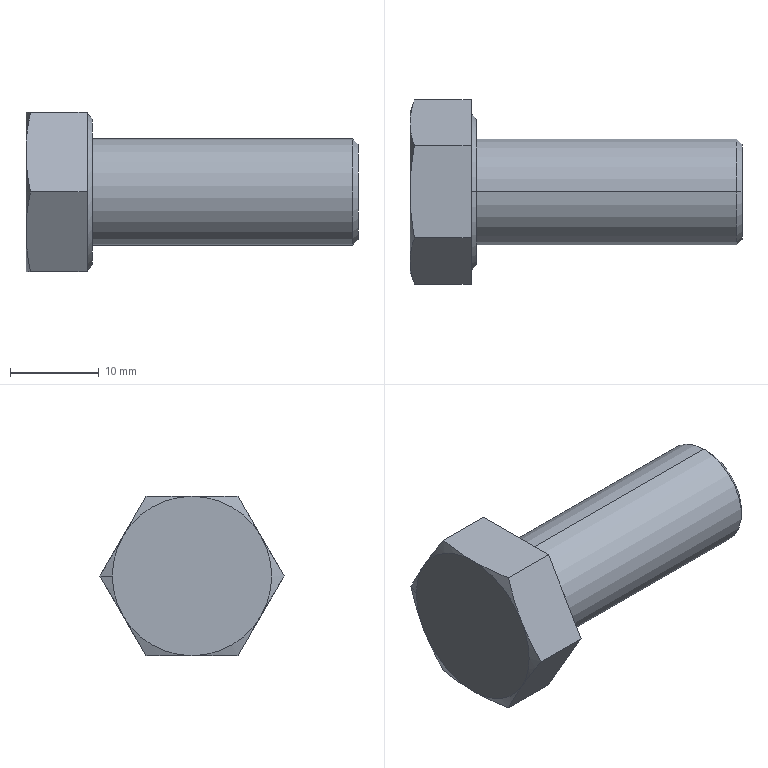Part | STEP file | hex head bolts-full thread grade c gb_GB_FASTENER_BOLT_HHBFTC M12X30-S | 1 solid | 23 faces | box 37.5 x 20.785 x 18 mm | volume 5456 mm3 | cone 11 | plane 10 | cylinder 2 | commonest cylinder face diameters 12 x2
STEP:
#1=CARTESIAN_POINT('',(36.9,0.,6.));
#2=VERTEX_POINT('',#1);
#3=CARTESIAN_POINT('',(36.9,0.,-6.));
#4=VERTEX_POINT('',#3);
#5=CARTESIAN_POINT('',(36.9,0.,0.));
#6=DIRECTION('',(-1.,0.,0.));
#7=DIRECTION('',(0.,0.,1.));
#8=AXIS2_PLACEMENT_3D('',#5,#6,#7);
#9=CIRCLE('',#8,6.);
#10=EDGE_CURVE('',#2,#4,#9,.T.);
#11=ORIENTED_EDGE('',*,*,#10,.T.);
#12=CARTESIAN_POINT('',(7.5,0.,-6.));
#13=VERTEX_POINT('',#12);
#14=CARTESIAN_POINT('',(37.5,0.,-6.));
#15=DIRECTION('',(-1.,0.,0.));
#16=VECTOR('',#15,1000.);
#17=LINE('',#14,#16);
#18=EDGE_CURVE('',#4,#13,#17,.T.);
#19=ORIENTED_EDGE('',*,*,#18,.T.);
#20=CARTESIAN_POINT('',(7.5,0.,6.));
#21=VERTEX_POINT('',#20);
#22=CARTESIAN_POINT('',(7.5,0.,0.));
#23=DIRECTION('',(1.,0.,0.));
#24=DIRECTION('',(0.,0.,1.));
#25=AXIS2_PLACEMENT_3D('',#22,#23,#24);
#26=CIRCLE('',#25,6.);
#27=EDGE_CURVE('',#13,#21,#26,.T.);
#28=ORIENTED_EDGE('',*,*,#27,.T.);
#29=CARTESIAN_POINT('',(37.5,0.,6.));
#30=DIRECTION('',(-1.,0.,0.));
#31=VECTOR('',#30,1000.);
#32=LINE('',#29,#31);
#33=EDGE_CURVE('',#2,#21,#32,.T.);
#34=ORIENTED_EDGE('',*,*,#33,.F.);
#35=EDGE_LOOP('',(#11,#19,#28,#34));
#36=FACE_OUTER_BOUND('',#35,.T.);
#37=CARTESIAN_POINT('',(37.5,0.,0.));
#38=DIRECTION('',(-1.,0.,0.));
#39=DIRECTION('',(0.,0.,1.));
#40=AXIS2_PLACEMENT_3D('',#37,#38,#39);
#41=CYLINDRICAL_SURFACE('',#40,6.);
#42=ADVANCED_FACE('',(#36),#41,.T.);
#43=CARTESIAN_POINT('',(37.5,0.,5.4));
#44=VERTEX_POINT('',#43);
#45=CARTESIAN_POINT('',(37.5,0.,-5.4));
#46=VERTEX_POINT('',#45);
#47=CARTESIAN_POINT('',(37.5,0.,0.));
#48=DIRECTION('',(-1.,0.,0.));
#49=DIRECTION('',(0.,0.,1.));
#50=AXIS2_PLACEMENT_3D('',#47,#48,#49);
#51=CIRCLE('',#50,5.4);
#52=EDGE_CURVE('',#44,#46,#51,.T.);
#53=ORIENTED_EDGE('',*,*,#52,.T.);
#54=CARTESIAN_POINT('',(36.9,0.,-6.));
#55=DIRECTION('',(-0.7071,0.,-0.7071));
#56=VECTOR('',#55,1000.);
#57=LINE('',#54,#56);
#58=EDGE_CURVE('',#46,#4,#57,.T.);
#59=ORIENTED_EDGE('',*,*,#58,.T.);
#60=ORIENTED_EDGE('',*,*,#10,.F.);
#61=CARTESIAN_POINT('',(36.9,0.,6.));
#62=DIRECTION('',(-0.7071,0.,0.7071));
#63=VECTOR('',#62,1000.);
#64=LINE('',#61,#63);
#65=EDGE_CURVE('',#44,#2,#64,.T.);
#66=ORIENTED_EDGE('',*,*,#65,.F.);
#67=EDGE_LOOP('',(#53,#59,#60,#66));
#68=FACE_OUTER_BOUND('',#67,.T.);
#69=CARTESIAN_POINT('',(36.9,0.,0.));
#70=DIRECTION('',(-1.,0.,0.));
#71=DIRECTION('',(0.,0.,1.));
#72=AXIS2_PLACEMENT_3D('',#69,#70,#71);
#73=CONICAL_SURFACE('',#72,6.,0.7854);
#74=ADVANCED_FACE('',(#68),#73,.T.);
#75=CARTESIAN_POINT('',(7.5,0.,8.235));
#76=VERTEX_POINT('',#75);
#77=CARTESIAN_POINT('',(7.5,0.,-8.235));
#78=VERTEX_POINT('',#77);
#79=CARTESIAN_POINT('',(7.5,0.,0.));
#80=DIRECTION('',(-1.,0.,0.));
#81=DIRECTION('',(0.,0.,1.));
#82=AXIS2_PLACEMENT_3D('',#79,#80,#81);
#83=CIRCLE('',#82,8.235);
#84=EDGE_CURVE('',#76,#78,#83,.T.);
#85=ORIENTED_EDGE('',*,*,#84,.T.);
#86=CARTESIAN_POINT('',(6.9,0.,-8.835));
#87=VERTEX_POINT('',#86);
#88=CARTESIAN_POINT('',(6.9,0.,-8.835));
#89=DIRECTION('',(-0.7071,0.,-0.7071));
#90=VECTOR('',#89,1000.);
#91=LINE('',#88,#90);
#92=EDGE_CURVE('',#78,#87,#91,.T.);
#93=ORIENTED_EDGE('',*,*,#92,.T.);
#94=CARTESIAN_POINT('',(6.9,0.,8.835));
#95=VERTEX_POINT('',#94);
#96=CARTESIAN_POINT('',(6.9,0.,0.));
#97=DIRECTION('',(1.,0.,0.));
#98=DIRECTION('',(0.,0.,1.));
#99=AXIS2_PLACEMENT_3D('',#96,#97,#98);
#100=CIRCLE('',#99,8.835);
#101=EDGE_CURVE('',#87,#95,#100,.T.);
#102=ORIENTED_EDGE('',*,*,#101,.T.);
#103=CARTESIAN_POINT('',(6.9,0.,8.835));
#104=DIRECTION('',(-0.7071,0.,0.7071));
#105=VECTOR('',#104,1000.);
#106=LINE('',#103,#105);
#107=EDGE_CURVE('',#76,#95,#106,.T.);
#108=ORIENTED_EDGE('',*,*,#107,.F.);
#109=EDGE_LOOP('',(#85,#93,#102,#108));
#110=FACE_OUTER_BOUND('',#109,.T.);
#111=CARTESIAN_POINT('',(6.9,0.,0.));
#112=DIRECTION('',(-1.,0.,0.));
#113=DIRECTION('',(0.,0.,1.));
#114=AXIS2_PLACEMENT_3D('',#111,#112,#113);
#115=CONICAL_SURFACE('',#114,8.835,0.7854);
#116=ADVANCED_FACE('',(#110),#115,.T.);
#117=CARTESIAN_POINT('',(0.,7.794,-4.5));
#118=VERTEX_POINT('',#117);
#119=CARTESIAN_POINT('',(0.,9.,0.));
#120=VERTEX_POINT('',#119);
#121=CARTESIAN_POINT('',(0.,0.,0.));
#122=DIRECTION('',(1.,0.,0.));
#123=DIRECTION('',(0.,1.,0.));
#124=AXIS2_PLACEMENT_3D('',#121,#122,#123);
#125=CIRCLE('',#124,9.);
#126=EDGE_CURVE('',#118,#120,#125,.T.);
#127=ORIENTED_EDGE('',*,*,#126,.T.);
#128=CARTESIAN_POINT('',(0.5068,10.392,0.));
#129=VERTEX_POINT('',#128);
#130=CARTESIAN_POINT('',(0.5098,10.401,0.));
#131=DIRECTION('',(0.342,0.9397,0.));
#132=VECTOR('',#131,1000.);
#133=LINE('',#130,#132);
#134=EDGE_CURVE('',#120,#129,#133,.T.);
#135=ORIENTED_EDGE('',*,*,#134,.T.);
#136=CARTESIAN_POINT('',(0.5068,10.392,0.));
#137=CARTESIAN_POINT('',(0.3504,9.963,-0.7439));
#138=CARTESIAN_POINT('',(0.2227,9.532,-1.49));
#139=CARTESIAN_POINT('',(0.04718,8.666,-2.99));
#140=CARTESIAN_POINT('',(0.,8.231,-3.743));
#141=CARTESIAN_POINT('',(0.,7.794,-4.5));
#142=B_SPLINE_CURVE_WITH_KNOTS('',3,(#136,#137,#138,#139,#140,#141),.UNSPECIFIED.,.F.,.F.,(4,2,4),(0.,0.00261,0.005221),.UNSPECIFIED.);
#143=EDGE_CURVE('',#129,#118,#142,.T.);
#144=ORIENTED_EDGE('',*,*,#143,.T.);
#145=EDGE_LOOP('',(#127,#135,#144));
#146=FACE_OUTER_BOUND('',#145,.T.);
#147=CARTESIAN_POINT('',(0.5098,0.,0.));
#148=DIRECTION('',(1.,0.,0.));
#149=DIRECTION('',(0.,1.,0.));
#150=AXIS2_PLACEMENT_3D('',#147,#148,#149);
#151=CONICAL_SURFACE('',#150,10.401,1.222);
#152=ADVANCED_FACE('',(#146),#151,.T.);
#153=ORIENTED_EDGE('',*,*,#18,.F.);
#154=CARTESIAN_POINT('',(36.9,0.,0.));
#155=DIRECTION('',(-1.,0.,0.));
#156=DIRECTION('',(0.,0.,1.));
#157=AXIS2_PLACEMENT_3D('',#154,#155,#156);
#158=CIRCLE('',#157,6.);
#159=EDGE_CURVE('',#4,#2,#158,.T.);
#160=ORIENTED_EDGE('',*,*,#159,.T.);
#161=ORIENTED_EDGE('',*,*,#33,.T.);
#162=CARTESIAN_POINT('',(7.5,0.,0.));
#163=DIRECTION('',(1.,0.,0.));
#164=DIRECTION('',(0.,0.,1.));
#165=AXIS2_PLACEMENT_3D('',#162,#163,#164);
#166=CIRCLE('',#165,6.);
#167=EDGE_CURVE('',#21,#13,#166,.T.);
#168=ORIENTED_EDGE('',*,*,#167,.T.);
#169=EDGE_LOOP('',(#153,#160,#161,#168));
#170=FACE_OUTER_BOUND('',#169,.T.);
#171=CARTESIAN_POINT('',(37.5,0.,0.));
#172=DIRECTION('',(-1.,0.,0.));
#173=DIRECTION('',(0.,0.,1.));
#174=AXIS2_PLACEMENT_3D('',#171,#172,#173);
#175=CYLINDRICAL_SURFACE('',#174,6.);
#176=ADVANCED_FACE('',(#170),#175,.T.);
#177=ORIENTED_EDGE('',*,*,#167,.F.);
#178=ORIENTED_EDGE('',*,*,#27,.F.);
#179=EDGE_LOOP('',(#177,#178));
#180=FACE_BOUND('',#179,.T.);
#181=ORIENTED_EDGE('',*,*,#84,.F.);
#182=CARTESIAN_POINT('',(7.5,0.,0.));
#183=DIRECTION('',(-1.,0.,0.));
#184=DIRECTION('',(0.,0.,1.));
#185=AXIS2_PLACEMENT_3D('',#182,#183,#184);
#186=CIRCLE('',#185,8.235);
#187=EDGE_CURVE('',#78,#76,#186,.T.);
#188=ORIENTED_EDGE('',*,*,#187,.F.);
#189=EDGE_LOOP('',(#181,#188));
#190=FACE_OUTER_BOUND('',#189,.T.);
#191=CARTESIAN_POINT('',(7.5,0.,18.));
#192=DIRECTION('',(-1.,0.,0.));
#193=DIRECTION('',(0.,0.,1.));
#194=AXIS2_PLACEMENT_3D('',#191,#192,#193);
#195=PLANE('',#194);
#196=ADVANCED_FACE('',(#180,#190),#195,.F.);
#197=ORIENTED_EDGE('',*,*,#58,.F.);
#198=CARTESIAN_POINT('',(37.5,0.,0.));
#199=DIRECTION('',(-1.,0.,0.));
#200=DIRECTION('',(0.,0.,1.));
#201=AXIS2_PLACEMENT_3D('',#198,#199,#200);
#202=CIRCLE('',#201,5.4);
#203=EDGE_CURVE('',#46,#44,#202,.T.);
#204=ORIENTED_EDGE('',*,*,#203,.T.);
#205=ORIENTED_EDGE('',*,*,#65,.T.);
#206=ORIENTED_EDGE('',*,*,#159,.F.);
#207=EDGE_LOOP('',(#197,#204,#205,#206));
#208=FACE_OUTER_BOUND('',#207,.T.);
#209=CARTESIAN_POINT('',(36.9,0.,0.));
#210=DIRECTION('',(-1.,0.,0.));
#211=DIRECTION('',(0.,0.,1.));
#212=AXIS2_PLACEMENT_3D('',#209,#210,#211);
#213=CONICAL_SURFACE('',#212,6.,0.7854);
#214=ADVANCED_FACE('',(#208),#213,.T.);
#215=ORIENTED_EDGE('',*,*,#92,.F.);
#216=ORIENTED_EDGE('',*,*,#187,.T.);
#217=ORIENTED_EDGE('',*,*,#107,.T.);
#218=CARTESIAN_POINT('',(6.9,0.,0.));
#219=DIRECTION('',(1.,0.,0.));
#220=DIRECTION('',(0.,0.,1.));
#221=AXIS2_PLACEMENT_3D('',#218,#219,#220);
#222=CIRCLE('',#221,8.835);
#223=EDGE_CURVE('',#95,#87,#222,.T.);
#224=ORIENTED_EDGE('',*,*,#223,.T.);
#225=EDGE_LOOP('',(#215,#216,#217,#224));
#226=FACE_OUTER_BOUND('',#225,.T.);
#227=CARTESIAN_POINT('',(6.9,0.,0.));
#228=DIRECTION('',(-1.,0.,0.));
#229=DIRECTION('',(0.,0.,1.));
#230=AXIS2_PLACEMENT_3D('',#227,#228,#229);
#231=CONICAL_SURFACE('',#230,8.835,0.7854);
#232=ADVANCED_FACE('',(#226),#231,.T.);
#233=ORIENTED_EDGE('',*,*,#52,.F.);
#234=ORIENTED_EDGE('',*,*,#203,.F.);
#235=EDGE_LOOP('',(#233,#234));
#236=FACE_OUTER_BOUND('',#235,.T.);
#237=CARTESIAN_POINT('',(37.5,0.,0.));
#238=DIRECTION('',(1.,0.,0.));
#239=DIRECTION('',(0.,0.,-1.));
#240=AXIS2_PLACEMENT_3D('',#237,#238,#239);
#241=PLANE('',#240);
#242=ADVANCED_FACE('',(#236),#241,.T.);
#243=CARTESIAN_POINT('',(6.9,10.392,0.));
#244=VERTEX_POINT('',#243);
#245=CARTESIAN_POINT('',(6.9,5.196,9.));
#246=VERTEX_POINT('',#245);
#247=CARTESIAN_POINT('',(6.9,10.392,0.));
#248=DIRECTION('',(0.,-0.5,0.866));
#249=VECTOR('',#248,1000.);
#250=LINE('',#247,#249);
#251=EDGE_CURVE('',#244,#246,#250,.T.);
#252=ORIENTED_EDGE('',*,*,#251,.T.);
#253=CARTESIAN_POINT('',(6.9,-5.196,9.));
#254=VERTEX_POINT('',#253);
#255=CARTESIAN_POINT('',(6.9,8.835,9.));
#256=DIRECTION('',(0.,-1.,0.));
#257=VECTOR('',#256,1000.);
#258=LINE('',#255,#257);
#259=EDGE_CURVE('',#246,#254,#258,.T.);
#260=ORIENTED_EDGE('',*,*,#259,.T.);
#261=CARTESIAN_POINT('',(6.9,-10.392,0.));
#262=VERTEX_POINT('',#261);
#263=CARTESIAN_POINT('',(6.9,-5.196,9.));
#264=DIRECTION('',(0.,-0.5,-0.866));
#265=VECTOR('',#264,1000.);
#266=LINE('',#263,#265);
#267=EDGE_CURVE('',#254,#262,#266,.T.);
#268=ORIENTED_EDGE('',*,*,#267,.T.);
#269=CARTESIAN_POINT('',(6.9,-5.196,-9.));
#270=VERTEX_POINT('',#269);
#271=CARTESIAN_POINT('',(6.9,-10.392,0.));
#272=DIRECTION('',(0.,0.5,-0.866));
#273=VECTOR('',#272,1000.);
#274=LINE('',#271,#273);
#275=EDGE_CURVE('',#262,#270,#274,.T.);
#276=ORIENTED_EDGE('',*,*,#275,.T.);
#277=CARTESIAN_POINT('',(6.9,5.196,-9.));
#278=VERTEX_POINT('',#277);
#279=CARTESIAN_POINT('',(6.9,8.835,-9.));
#280=DIRECTION('',(0.,1.,0.));
#281=VECTOR('',#280,1000.);
#282=LINE('',#279,#281);
#283=EDGE_CURVE('',#270,#278,#282,.T.);
#284=ORIENTED_EDGE('',*,*,#283,.T.);
#285=CARTESIAN_POINT('',(6.9,5.196,-9.));
#286=DIRECTION('',(0.,0.5,0.866));
#287=VECTOR('',#286,1000.);
#288=LINE('',#285,#287);
#289=EDGE_CURVE('',#278,#244,#288,.T.);
#290=ORIENTED_EDGE('',*,*,#289,.T.);
#291=EDGE_LOOP('',(#252,#260,#268,#276,#284,#290));
#292=FACE_OUTER_BOUND('',#291,.T.);
#293=ORIENTED_EDGE('',*,*,#223,.F.);
#294=ORIENTED_EDGE('',*,*,#101,.F.);
#295=EDGE_LOOP('',(#293,#294));
#296=FACE_BOUND('',#295,.T.);
#297=CARTESIAN_POINT('',(6.9,8.835,0.));
#298=DIRECTION('',(1.,0.,0.));
#299=DIRECTION('',(0.,0.,-1.));
#300=AXIS2_PLACEMENT_3D('',#297,#298,#299);
#301=PLANE('',#300);
#302=ADVANCED_FACE('',(#292,#296),#301,.T.);
#303=CARTESIAN_POINT('',(0.5068,-5.196,9.));
#304=VERTEX_POINT('',#303);
#305=CARTESIAN_POINT('',(7.5,-5.196,9.));
#306=DIRECTION('',(-1.,0.,0.));
#307=VECTOR('',#306,1000.);
#308=LINE('',#305,#307);
#309=EDGE_CURVE('',#254,#304,#308,.T.);
#310=ORIENTED_EDGE('',*,*,#309,.F.);
#311=ORIENTED_EDGE('',*,*,#259,.F.);
#312=CARTESIAN_POINT('',(0.5068,5.196,9.));
#313=VERTEX_POINT('',#312);
#314=CARTESIAN_POINT('',(7.5,5.196,9.));
#315=DIRECTION('',(1.,0.,0.));
#316=VECTOR('',#315,1000.);
#317=LINE('',#314,#316);
#318=EDGE_CURVE('',#313,#246,#317,.T.);
#319=ORIENTED_EDGE('',*,*,#318,.F.);
#320=CARTESIAN_POINT('',(0.,0.,9.));
#321=VERTEX_POINT('',#320);
#322=CARTESIAN_POINT('',(0.,0.,9.));
#323=CARTESIAN_POINT('',(0.,0.8743,9.));
#324=CARTESIAN_POINT('',(0.04718,1.744,9.));
#325=CARTESIAN_POINT('',(0.2227,3.475,9.));
#326=CARTESIAN_POINT('',(0.3504,4.337,9.));
#327=CARTESIAN_POINT('',(0.5068,5.196,9.));
#328=B_SPLINE_CURVE_WITH_KNOTS('',3,(#322,#323,#324,#325,#326,#327),.UNSPECIFIED.,.F.,.F.,(4,2,4),(0.,0.00261,0.005221),.UNSPECIFIED.);
#329=EDGE_CURVE('',#321,#313,#328,.T.);
#330=ORIENTED_EDGE('',*,*,#329,.F.);
#331=CARTESIAN_POINT('',(0.5068,-5.196,9.));
#332=CARTESIAN_POINT('',(0.3504,-4.337,9.));
#333=CARTESIAN_POINT('',(0.2227,-3.475,9.));
#334=CARTESIAN_POINT('',(0.04718,-1.744,9.));
#335=CARTESIAN_POINT('',(0.,-0.8743,9.));
#336=CARTESIAN_POINT('',(0.,0.,9.));
#337=B_SPLINE_CURVE_WITH_KNOTS('',3,(#331,#332,#333,#334,#335,#336),.UNSPECIFIED.,.F.,.F.,(4,2,4),(0.,0.00261,0.005221),.UNSPECIFIED.);
#338=EDGE_CURVE('',#304,#321,#337,.T.);
#339=ORIENTED_EDGE('',*,*,#338,.F.);
#340=EDGE_LOOP('',(#310,#311,#319,#330,#339));
#341=FACE_OUTER_BOUND('',#340,.T.);
#342=CARTESIAN_POINT('',(7.5,5.196,9.));
#343=DIRECTION('',(0.,0.,-1.));
#344=DIRECTION('',(-1.,0.,0.));
#345=AXIS2_PLACEMENT_3D('',#342,#343,#344);
#346=PLANE('',#345);
#347=ADVANCED_FACE('',(#341),#346,.F.);
#348=ORIENTED_EDGE('',*,*,#318,.T.);
#349=ORIENTED_EDGE('',*,*,#251,.F.);
#350=CARTESIAN_POINT('',(7.5,10.392,0.));
#351=DIRECTION('',(1.,0.,0.));
#352=VECTOR('',#351,1000.);
#353=LINE('',#350,#352);
#354=EDGE_CURVE('',#129,#244,#353,.T.);
#355=ORIENTED_EDGE('',*,*,#354,.F.);
#356=CARTESIAN_POINT('',(0.,7.794,4.5));
#357=VERTEX_POINT('',#356);
#358=CARTESIAN_POINT('',(0.,7.794,4.5));
#359=CARTESIAN_POINT('',(0.,8.231,3.743));
#360=CARTESIAN_POINT('',(0.04718,8.666,2.99));
#361=CARTESIAN_POINT('',(0.2227,9.532,1.49));
#362=CARTESIAN_POINT('',(0.3504,9.963,0.7439));
#363=CARTESIAN_POINT('',(0.5068,10.392,0.));
#364=B_SPLINE_CURVE_WITH_KNOTS('',3,(#358,#359,#360,#361,#362,#363),.UNSPECIFIED.,.F.,.F.,(4,2,4),(0.,0.00261,0.005221),.UNSPECIFIED.);
#365=EDGE_CURVE('',#357,#129,#364,.T.);
#366=ORIENTED_EDGE('',*,*,#365,.F.);
#367=CARTESIAN_POINT('',(0.5068,5.196,9.));
#368=CARTESIAN_POINT('',(0.3504,5.626,8.256));
#369=CARTESIAN_POINT('',(0.2227,6.057,7.51));
#370=CARTESIAN_POINT('',(0.04718,6.922,6.01));
#371=CARTESIAN_POINT('',(0.,7.357,5.257));
#372=CARTESIAN_POINT('',(0.,7.794,4.5));
#373=B_SPLINE_CURVE_WITH_KNOTS('',3,(#367,#368,#369,#370,#371,#372),.UNSPECIFIED.,.F.,.F.,(4,2,4),(0.,0.00261,0.005221),.UNSPECIFIED.);
#374=EDGE_CURVE('',#313,#357,#373,.T.);
#375=ORIENTED_EDGE('',*,*,#374,.F.);
#376=EDGE_LOOP('',(#348,#349,#355,#366,#375));
#377=FACE_OUTER_BOUND('',#376,.T.);
#378=CARTESIAN_POINT('',(7.5,10.392,0.));
#379=DIRECTION('',(0.,-0.866,-0.5));
#380=DIRECTION('',(0.,0.5,-0.866));
#381=AXIS2_PLACEMENT_3D('',#378,#379,#380);
#382=PLANE('',#381);
#383=ADVANCED_FACE('',(#377),#382,.F.);
#384=ORIENTED_EDGE('',*,*,#354,.T.);
#385=ORIENTED_EDGE('',*,*,#289,.F.);
#386=CARTESIAN_POINT('',(0.5068,5.196,-9.));
#387=VERTEX_POINT('',#386);
#388=CARTESIAN_POINT('',(7.5,5.196,-9.));
#389=DIRECTION('',(1.,0.,0.));
#390=VECTOR('',#389,1000.);
#391=LINE('',#388,#390);
#392=EDGE_CURVE('',#387,#278,#391,.T.);
#393=ORIENTED_EDGE('',*,*,#392,.F.);
#394=CARTESIAN_POINT('',(0.,7.794,-4.5));
#395=CARTESIAN_POINT('',(0.,7.357,-5.257));
#396=CARTESIAN_POINT('',(0.04718,6.922,-6.01));
#397=CARTESIAN_POINT('',(0.2227,6.057,-7.51));
#398=CARTESIAN_POINT('',(0.3504,5.626,-8.256));
#399=CARTESIAN_POINT('',(0.5068,5.196,-9.));
#400=B_SPLINE_CURVE_WITH_KNOTS('',3,(#394,#395,#396,#397,#398,#399),.UNSPECIFIED.,.F.,.F.,(4,2,4),(0.,0.00261,0.005221),.UNSPECIFIED.);
#401=EDGE_CURVE('',#118,#387,#400,.T.);
#402=ORIENTED_EDGE('',*,*,#401,.F.);
#403=ORIENTED_EDGE('',*,*,#143,.F.);
#404=EDGE_LOOP('',(#384,#385,#393,#402,#403));
#405=FACE_OUTER_BOUND('',#404,.T.);
#406=CARTESIAN_POINT('',(7.5,5.196,-9.));
#407=DIRECTION('',(0.,-0.866,0.5));
#408=DIRECTION('',(0.,-0.5,-0.866));
#409=AXIS2_PLACEMENT_3D('',#406,#407,#408);
#410=PLANE('',#409);
#411=ADVANCED_FACE('',(#405),#410,.F.);
#412=ORIENTED_EDGE('',*,*,#392,.T.);
#413=ORIENTED_EDGE('',*,*,#283,.F.);
#414=CARTESIAN_POINT('',(0.5068,-5.196,-9.));
#415=VERTEX_POINT('',#414);
#416=CARTESIAN_POINT('',(7.5,-5.196,-9.));
#417=DIRECTION('',(1.,0.,0.));
#418=VECTOR('',#417,1000.);
#419=LINE('',#416,#418);
#420=EDGE_CURVE('',#415,#270,#419,.T.);
#421=ORIENTED_EDGE('',*,*,#420,.F.);
#422=CARTESIAN_POINT('',(0.,0.,-9.));
#423=VERTEX_POINT('',#422);
#424=CARTESIAN_POINT('',(0.,0.,-9.));
#425=CARTESIAN_POINT('',(0.,-0.8743,-9.));
#426=CARTESIAN_POINT('',(0.04718,-1.744,-9.));
#427=CARTESIAN_POINT('',(0.2227,-3.475,-9.));
#428=CARTESIAN_POINT('',(0.3504,-4.337,-9.));
#429=CARTESIAN_POINT('',(0.5068,-5.196,-9.));
#430=B_SPLINE_CURVE_WITH_KNOTS('',3,(#424,#425,#426,#427,#428,#429),.UNSPECIFIED.,.F.,.F.,(4,2,4),(0.,0.00261,0.005221),.UNSPECIFIED.);
#431=EDGE_CURVE('',#423,#415,#430,.T.);
#432=ORIENTED_EDGE('',*,*,#431,.F.);
#433=CARTESIAN_POINT('',(0.5068,5.196,-9.));
#434=CARTESIAN_POINT('',(0.3504,4.337,-9.));
#435=CARTESIAN_POINT('',(0.2227,3.475,-9.));
#436=CARTESIAN_POINT('',(0.04718,1.744,-9.));
#437=CARTESIAN_POINT('',(0.,0.8743,-9.));
#438=CARTESIAN_POINT('',(0.,0.,-9.));
#439=B_SPLINE_CURVE_WITH_KNOTS('',3,(#433,#434,#435,#436,#437,#438),.UNSPECIFIED.,.F.,.F.,(4,2,4),(0.,0.00261,0.005221),.UNSPECIFIED.);
#440=EDGE_CURVE('',#387,#423,#439,.T.);
#441=ORIENTED_EDGE('',*,*,#440,.F.);
#442=EDGE_LOOP('',(#412,#413,#421,#432,#441));
#443=FACE_OUTER_BOUND('',#442,.T.);
#444=CARTESIAN_POINT('',(7.5,-5.196,-9.));
#445=DIRECTION('',(0.,0.,1.));
#446=DIRECTION('',(1.,0.,0.));
#447=AXIS2_PLACEMENT_3D('',#444,#445,#446);
#448=PLANE('',#447);
#449=ADVANCED_FACE('',(#443),#448,.F.);
#450=ORIENTED_EDGE('',*,*,#420,.T.);
#451=ORIENTED_EDGE('',*,*,#275,.F.);
#452=CARTESIAN_POINT('',(0.5068,-10.392,0.));
#453=VERTEX_POINT('',#452);
#454=CARTESIAN_POINT('',(7.5,-10.392,0.));
#455=DIRECTION('',(1.,0.,0.));
#456=VECTOR('',#455,1000.);
#457=LINE('',#454,#456);
#458=EDGE_CURVE('',#453,#262,#457,.T.);
#459=ORIENTED_EDGE('',*,*,#458,.F.);
#460=CARTESIAN_POINT('',(0.,-7.794,-4.5));
#461=VERTEX_POINT('',#460);
#462=CARTESIAN_POINT('',(0.,-7.794,-4.5));
#463=CARTESIAN_POINT('',(0.,-8.231,-3.743));
#464=CARTESIAN_POINT('',(0.04718,-8.666,-2.99));
#465=CARTESIAN_POINT('',(0.2227,-9.532,-1.49));
#466=CARTESIAN_POINT('',(0.3504,-9.963,-0.7439));
#467=CARTESIAN_POINT('',(0.5068,-10.392,0.));
#468=B_SPLINE_CURVE_WITH_KNOTS('',3,(#462,#463,#464,#465,#466,#467),.UNSPECIFIED.,.F.,.F.,(4,2,4),(0.,0.00261,0.005221),.UNSPECIFIED.);
#469=EDGE_CURVE('',#461,#453,#468,.T.);
#470=ORIENTED_EDGE('',*,*,#469,.F.);
#471=CARTESIAN_POINT('',(0.5068,-5.196,-9.));
#472=CARTESIAN_POINT('',(0.3504,-5.626,-8.256));
#473=CARTESIAN_POINT('',(0.2227,-6.057,-7.51));
#474=CARTESIAN_POINT('',(0.04718,-6.922,-6.01));
#475=CARTESIAN_POINT('',(0.,-7.357,-5.257));
#476=CARTESIAN_POINT('',(0.,-7.794,-4.5));
#477=B_SPLINE_CURVE_WITH_KNOTS('',3,(#471,#472,#473,#474,#475,#476),.UNSPECIFIED.,.F.,.F.,(4,2,4),(0.,0.00261,0.005221),.UNSPECIFIED.);
#478=EDGE_CURVE('',#415,#461,#477,.T.);
#479=ORIENTED_EDGE('',*,*,#478,.F.);
#480=EDGE_LOOP('',(#450,#451,#459,#470,#479));
#481=FACE_OUTER_BOUND('',#480,.T.);
#482=CARTESIAN_POINT('',(7.5,-10.392,0.));
#483=DIRECTION('',(0.,0.866,0.5));
#484=DIRECTION('',(0.,-0.5,0.866));
#485=AXIS2_PLACEMENT_3D('',#482,#483,#484);
#486=PLANE('',#485);
#487=ADVANCED_FACE('',(#481),#486,.F.);
#488=ORIENTED_EDGE('',*,*,#458,.T.);
#489=ORIENTED_EDGE('',*,*,#267,.F.);
#490=ORIENTED_EDGE('',*,*,#309,.T.);
#491=CARTESIAN_POINT('',(0.,-7.794,4.5));
#492=VERTEX_POINT('',#491);
#493=CARTESIAN_POINT('',(0.,-7.794,4.5));
#494=CARTESIAN_POINT('',(0.,-7.357,5.257));
#495=CARTESIAN_POINT('',(0.04718,-6.922,6.01));
#496=CARTESIAN_POINT('',(0.2227,-6.057,7.51));
#497=CARTESIAN_POINT('',(0.3504,-5.626,8.256));
#498=CARTESIAN_POINT('',(0.5068,-5.196,9.));
#499=B_SPLINE_CURVE_WITH_KNOTS('',3,(#493,#494,#495,#496,#497,#498),.UNSPECIFIED.,.F.,.F.,(4,2,4),(0.,0.00261,0.005221),.UNSPECIFIED.);
#500=EDGE_CURVE('',#492,#304,#499,.T.);
#501=ORIENTED_EDGE('',*,*,#500,.F.);
#502=CARTESIAN_POINT('',(0.5068,-10.392,0.));
#503=CARTESIAN_POINT('',(0.3504,-9.963,0.7439));
#504=CARTESIAN_POINT('',(0.2227,-9.532,1.49));
#505=CARTESIAN_POINT('',(0.04718,-8.666,2.99));
#506=CARTESIAN_POINT('',(0.,-8.231,3.743));
#507=CARTESIAN_POINT('',(0.,-7.794,4.5));
#508=B_SPLINE_CURVE_WITH_KNOTS('',3,(#502,#503,#504,#505,#506,#507),.UNSPECIFIED.,.F.,.F.,(4,2,4),(0.,0.00261,0.005221),.UNSPECIFIED.);
#509=EDGE_CURVE('',#453,#492,#508,.T.);
#510=ORIENTED_EDGE('',*,*,#509,.F.);
#511=EDGE_LOOP('',(#488,#489,#490,#501,#510));
#512=FACE_OUTER_BOUND('',#511,.T.);
#513=CARTESIAN_POINT('',(7.5,-5.196,9.));
#514=DIRECTION('',(0.,0.866,-0.5));
#515=DIRECTION('',(0.,0.5,0.866));
#516=AXIS2_PLACEMENT_3D('',#513,#514,#515);
#517=PLANE('',#516);
#518=ADVANCED_FACE('',(#512),#517,.F.);
#519=ORIENTED_EDGE('',*,*,#338,.T.);
#520=CARTESIAN_POINT('',(0.,0.,0.));
#521=DIRECTION('',(1.,0.,0.));
#522=DIRECTION('',(0.,1.,0.));
#523=AXIS2_PLACEMENT_3D('',#520,#521,#522);
#524=CIRCLE('',#523,9.);
#525=EDGE_CURVE('',#321,#492,#524,.T.);
#526=ORIENTED_EDGE('',*,*,#525,.T.);
#527=ORIENTED_EDGE('',*,*,#500,.T.);
#528=EDGE_LOOP('',(#519,#526,#527));
#529=FACE_OUTER_BOUND('',#528,.T.);
#530=CARTESIAN_POINT('',(0.5098,0.,0.));
#531=DIRECTION('',(1.,0.,0.));
#532=DIRECTION('',(0.,1.,0.));
#533=AXIS2_PLACEMENT_3D('',#530,#531,#532);
#534=CONICAL_SURFACE('',#533,10.401,1.222);
#535=ADVANCED_FACE('',(#529),#534,.T.);
#536=CARTESIAN_POINT('',(0.,0.,0.));
#537=DIRECTION('',(1.,0.,0.));
#538=DIRECTION('',(0.,1.,0.));
#539=AXIS2_PLACEMENT_3D('',#536,#537,#538);
#540=CIRCLE('',#539,9.);
#541=EDGE_CURVE('',#357,#321,#540,.T.);
#542=ORIENTED_EDGE('',*,*,#541,.T.);
#543=ORIENTED_EDGE('',*,*,#329,.T.);
#544=ORIENTED_EDGE('',*,*,#374,.T.);
#545=EDGE_LOOP('',(#542,#543,#544));
#546=FACE_OUTER_BOUND('',#545,.T.);
#547=CARTESIAN_POINT('',(0.5098,0.,0.));
#548=DIRECTION('',(1.,0.,0.));
#549=DIRECTION('',(0.,1.,0.));
#550=AXIS2_PLACEMENT_3D('',#547,#548,#549);
#551=CONICAL_SURFACE('',#550,10.401,1.222);
#552=ADVANCED_FACE('',(#546),#551,.T.);
#553=ORIENTED_EDGE('',*,*,#134,.F.);
#554=CARTESIAN_POINT('',(0.,0.,0.));
#555=DIRECTION('',(1.,0.,0.));
#556=DIRECTION('',(0.,1.,0.));
#557=AXIS2_PLACEMENT_3D('',#554,#555,#556);
#558=CIRCLE('',#557,9.);
#559=EDGE_CURVE('',#120,#357,#558,.T.);
#560=ORIENTED_EDGE('',*,*,#559,.T.);
#561=ORIENTED_EDGE('',*,*,#365,.T.);
#562=EDGE_LOOP('',(#553,#560,#561));
#563=FACE_OUTER_BOUND('',#562,.T.);
#564=CARTESIAN_POINT('',(0.5098,0.,0.));
#565=DIRECTION('',(1.,0.,0.));
#566=DIRECTION('',(0.,1.,0.));
#567=AXIS2_PLACEMENT_3D('',#564,#565,#566);
#568=CONICAL_SURFACE('',#567,10.401,1.222);
#569=ADVANCED_FACE('',(#563),#568,.T.);
#570=CARTESIAN_POINT('',(0.,0.,0.));
#571=DIRECTION('',(1.,0.,0.));
#572=DIRECTION('',(0.,1.,0.));
#573=AXIS2_PLACEMENT_3D('',#570,#571,#572);
#574=CIRCLE('',#573,9.);
#575=EDGE_CURVE('',#423,#118,#574,.T.);
#576=ORIENTED_EDGE('',*,*,#575,.T.);
#577=ORIENTED_EDGE('',*,*,#401,.T.);
#578=ORIENTED_EDGE('',*,*,#440,.T.);
#579=EDGE_LOOP('',(#576,#577,#578));
#580=FACE_OUTER_BOUND('',#579,.T.);
#581=CARTESIAN_POINT('',(0.5098,0.,0.));
#582=DIRECTION('',(1.,0.,0.));
#583=DIRECTION('',(0.,1.,0.));
#584=AXIS2_PLACEMENT_3D('',#581,#582,#583);
#585=CONICAL_SURFACE('',#584,10.401,1.222);
#586=ADVANCED_FACE('',(#580),#585,.T.);
#587=ORIENTED_EDGE('',*,*,#478,.T.);
#588=CARTESIAN_POINT('',(0.,0.,0.));
#589=DIRECTION('',(1.,0.,0.));
#590=DIRECTION('',(0.,0.,-1.));
#591=AXIS2_PLACEMENT_3D('',#588,#589,#590);
#592=CIRCLE('',#591,9.);
#593=EDGE_CURVE('',#461,#423,#592,.T.);
#594=ORIENTED_EDGE('',*,*,#593,.T.);
#595=ORIENTED_EDGE('',*,*,#431,.T.);
#596=EDGE_LOOP('',(#587,#594,#595));
#597=FACE_OUTER_BOUND('',#596,.T.);
#598=CARTESIAN_POINT('',(0.5098,0.,0.));
#599=DIRECTION('',(1.,0.,0.));
#600=DIRECTION('',(0.,0.,-1.));
#601=AXIS2_PLACEMENT_3D('',#598,#599,#600);
#602=CONICAL_SURFACE('',#601,10.401,1.222);
#603=ADVANCED_FACE('',(#597),#602,.T.);
#604=ORIENTED_EDGE('',*,*,#509,.T.);
#605=CARTESIAN_POINT('',(0.,0.,0.));
#606=DIRECTION('',(1.,0.,0.));
#607=DIRECTION('',(0.,1.,0.));
#608=AXIS2_PLACEMENT_3D('',#605,#606,#607);
#609=CIRCLE('',#608,9.);
#610=EDGE_CURVE('',#492,#461,#609,.T.);
#611=ORIENTED_EDGE('',*,*,#610,.T.);
#612=ORIENTED_EDGE('',*,*,#469,.T.);
#613=EDGE_LOOP('',(#604,#611,#612));
#614=FACE_OUTER_BOUND('',#613,.T.);
#615=CARTESIAN_POINT('',(0.5098,0.,0.));
#616=DIRECTION('',(1.,0.,0.));
#617=DIRECTION('',(0.,1.,0.));
#618=AXIS2_PLACEMENT_3D('',#615,#616,#617);
#619=CONICAL_SURFACE('',#618,10.401,1.222);
#620=ADVANCED_FACE('',(#614),#619,.T.);
#621=ORIENTED_EDGE('',*,*,#593,.F.);
#622=ORIENTED_EDGE('',*,*,#610,.F.);
#623=ORIENTED_EDGE('',*,*,#525,.F.);
#624=ORIENTED_EDGE('',*,*,#541,.F.);
#625=ORIENTED_EDGE('',*,*,#559,.F.);
#626=ORIENTED_EDGE('',*,*,#126,.F.);
#627=ORIENTED_EDGE('',*,*,#575,.F.);
#628=EDGE_LOOP('',(#621,#622,#623,#624,#625,#626,#627));
#629=FACE_OUTER_BOUND('',#628,.T.);
#630=CARTESIAN_POINT('',(0.,0.,18.));
#631=DIRECTION('',(-1.,0.,0.));
#632=DIRECTION('',(0.,0.,1.));
#633=AXIS2_PLACEMENT_3D('',#630,#631,#632);
#634=PLANE('',#633);
#635=ADVANCED_FACE('',(#629),#634,.T.);
#636=CLOSED_SHELL('',(#42,#74,#116,#152,#176,#196,#214,#232,#242,#302,#347,#383,#411,#449,#487,#518,#535,#552,#569,#586,#603,#620,#635));
#637=MANIFOLD_SOLID_BREP('',#636);
#638=CARTESIAN_POINT('',(0.,0.,0.));
#639=DIRECTION('',(0.,0.,1.));
#640=DIRECTION('',(1.,0.,0.));
#641=AXIS2_PLACEMENT_3D('',#638,#639,#640);
#642=(LENGTH_UNIT()NAMED_UNIT(*)SI_UNIT(.MILLI.,.METRE.));
#643=UNCERTAINTY_MEASURE_WITH_UNIT(LENGTH_MEASURE(0.00001),#642,'','');
#644=(NAMED_UNIT(*)PLANE_ANGLE_UNIT()SI_UNIT($,.RADIAN.));
#645=(NAMED_UNIT(*)SI_UNIT($,.STERADIAN.)SOLID_ANGLE_UNIT());
#646=(GEOMETRIC_REPRESENTATION_CONTEXT(3)GLOBAL_UNCERTAINTY_ASSIGNED_CONTEXT((#643))GLOBAL_UNIT_ASSIGNED_CONTEXT((#642,#644,#645))REPRESENTATION_CONTEXT('',''));
#647=ADVANCED_BREP_SHAPE_REPRESENTATION('',(#637,#641),#646);